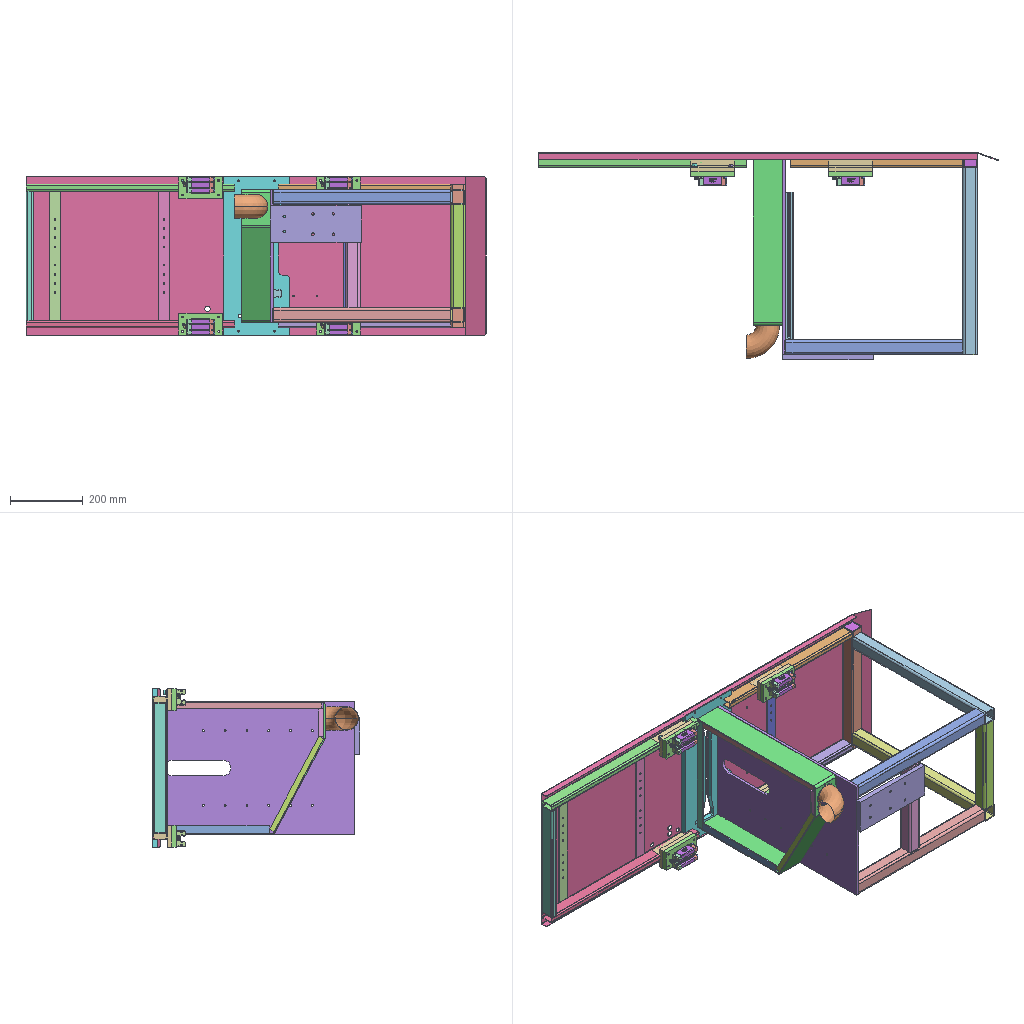Assembly | SolidWorks | 13 different items | 23 placed | box 1267 x 570 x 440 mm
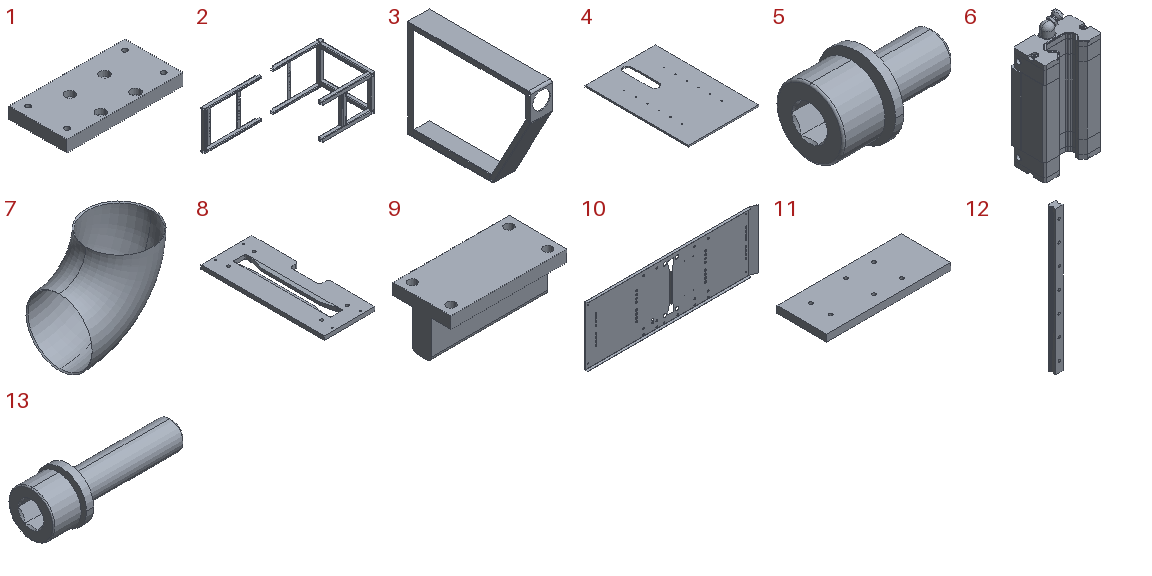Parts list (item | quantity | size | volume | features):
1 | x4 | 120 x 60 x 12 mm | 83068 mm3 | features HoleWzd 2, 3DProfileFeature 1, Extrusion 1
2 | x1 | 1210 x 555 x 396 mm | 2067194 mm3 | features ICE 3, WeldMemberFeat 3, WeldCornerFeat 2, 3DProfileFeature 1, EndCap 1, HoleWzd 1, WeldmentFeature 1
3 | x1 | 80 x 460 x 365 mm | 345434 mm3 | features ICE 3, FlatPattern 1, SMBaseFlange 1, SheetMetal 1
4 | x1 | 365 x 540 x 8 mm | 1513471 mm3 | features Extrusion 1, HoleWzd 1, LPattern 1
5 | x1 | 24 x 15 x 15 mm | 1870 mm3 | features RevCut 2, Revolution 2, Chamfer 1, Cut 1, Fillet 1
6 | x4 | 44.1 x 25.7 x 88.625 mm | 65252 mm3 | features ICE 20, Extrusion 4, MirrorPattern 4, Chamfer 3, Fillet 3, MirrorSolid 3, Revolution 2, Dome 1, RevCut 1
7 | x1 | 91.534 x 65 x 91.534 mm | 19075 mm3 | features Chamfer 1, Revolution 1
8 | x1 | 180 x 436 x 14 mm | 907497 mm3 | features HoleWzd 2, ICE 2, Extrusion 1, Fillet 1
9 | x4 | 120 x 60 x 52 mm | 178059 mm3 | features Extrusion 1, Fillet 1, HoleWzd 1, ICE 1
10 | x1 | 1267 x 21.649 x 440.4 mm | 706056 mm3 | features EdgeFlange 3, HoleWzd 3, LPattern 3, Fillet 2, ICE 2, FlatPattern 1, SMBaseFlange 1, SheetMetal 1
11 | x1 | 250 x 100 x 14 mm | 346949 mm3 | features HoleWzd 2, Extrusion 1
12 | x2 | 23 x 22 x 420 mm | 180087 mm3 | features ICE 17, Chamfer 3, Extrusion 3, Fillet 3, MirrorPattern 3, MirrorSolid 3, RevCut 2, DeleteBody 1, Dome 1, LPattern 1
13 | x1 | 31 x 11 x 11 mm | 1178 mm3 | features RevCut 2, Revolution 2, Chamfer 1, Cut 1, Fillet 1
Mates (type | each side: item.copy, entity, surface, feature):
DistanceDim | 9.1 face plane Boss-Extrude1 | 9.2 face plane Boss-Extrude1
Coincident | 2.1 face plane Cut-Extrude2 | 8.1 face plane Boss-Extrude1 | 2 times
Coincident | 8.1 face plane Boss-Extrude1 | 4.1 face plane Boss-Extrude1
Coincident | 9.1 face plane Boss-Extrude1 | 9.3 face plane Boss-Extrude1 | 2 times
Coincident | 4.1 face plane Boss-Extrude1 | 3.1 face plane Base-Flange1 | 2 times
Coincident | 8.1 face plane Boss-Extrude1 | 3.1 face plane Base-Flange1
DistanceDim | 3.1 face plane Base-Flange1 | 7.1 plane
Coincident | 2.1 face plane Square Tube 40 X 40 X 3.2(1) | 11.1 face plane Boss-Extrude1
Coincident | 4.1 face plane Boss-Extrude1 | 11.1 face plane Boss-Extrude1
DistanceDim | 11.1 face plane Boss-Extrude1 | 2.1 face plane Square Tube 40 X 40 X 3.2(1)
Concentric | assembly face | 1.1 face cylinder Hole Size (per hex socket screw type)1
Concentric | assembly face | 1.1 edge
Coincident | assembly face | 1.1 face plane Boss-Extrude1
Coincident | 9.3 face plane Boss-Extrude1 | 1.1 face plane Boss-Extrude1 | 3 times
Concentric | assembly face | 1.2 edge
Concentric | assembly edge | 1.2 face cylinder Hole Size (per hex socket screw type)1
Coincident | assembly face | 1.2 face plane Boss-Extrude1
Coincident | 9.1 face plane Boss-Extrude1 | 1.2 face plane Boss-Extrude1 | 3 times
Coincident | 9.2 face plane Boss-Extrude1 | 1.3 face plane Boss-Extrude1 | 3 times
Coincident | 9.4 face plane Boss-Extrude1 | 1.4 face plane Boss-Extrude1 | 3 times
Coincident | 8.1 face plane Boss-Extrude1 | 10.1 face plane Base-Flange1
Coincident | 4.1 face plane Boss-Extrude1 | 12.1 face plane Boss-Extrude8
Width | 3.1 face plane Base-Flange1 | 3.1 face plane Base-Flange1 | 8.1 face plane Boss-Extrude1 | 8.1 face plane Boss-Extrude1
Coincident | 1.4 face plane Boss-Extrude1 | 1.3 face plane Boss-Extrude1
Coincident | 9.1 face plane Boss-Extrude1 | 9.2 face plane Boss-Extrude1
Concentric | 1.1 edge | 6.1 face cylinder Cut-Revolve1
Concentric | 1.1 face cylinder Hole Size (per hex socket screw type)1 | 6.1 face cylinder Mirror1
Coincident | 1.1 face plane Boss-Extrude1 | 6.1 face plane Boss-Extrude1
Concentric | 1.2 edge | 6.2 face cylinder Cut-Revolve1
Concentric | 1.2 face cylinder Hole Size (per hex socket screw type)1 | 6.2 face cylinder Mirror2
Coincident | 1.2 face plane Boss-Extrude1 | 6.2 face plane Boss-Extrude1
Concentric | 1.3 face cylinder Hole Size (per hex socket screw type)1 | 6.3 face cylinder Mirror2
Concentric | 1.3 edge | 6.3 face cylinder Cut-Revolve1
Coincident | 1.3 face plane Boss-Extrude1 | 6.3 face plane Boss-Extrude1
Concentric | 1.4 face cylinder Hole Size (per hex socket screw type)1 | 6.4 face cylinder Cut-Revolve1
Concentric | 1.4 face cylinder Hole Size (per hex socket screw type)1 | 6.4 face cylinder Mirror1
Coincident | 1.4 face plane Boss-Extrude1 | 6.4 face plane Boss-Extrude1
Coincident | 9.4 face plane Boss-Extrude1 | 9.3 face plane Boss-Extrude1 | 2 times
Concentric | 4.1 face cylinder LPattern1 | 12.1 face cylinder LPattern1
Concentric | 4.1 face cylinder LPattern1 | 12.2 face cylinder LPattern1
Width | 8.1 face plane Boss-Extrude1 | 8.1 face plane Boss-Extrude1 | 2.1 face plane Rect Tube 40X20X2.5(6) | 2.1 face plane Rect Tube 40X20X2.5(6)
DistanceDim | 4.1 face plane Boss-Extrude1 | 8.1 face plane Boss-Extrude1
Coincident | 2.1 face plane Rect Tube 40X20X2.5(6) | 9.1 face plane Boss-Extrude2
Coincident | 2.1 face plane Rect Tube 40X20X2.5(6) | 9.3 face plane Boss-Extrude2
Coincident | 9.4 face plane Boss-Extrude1 | 9.2 face plane Boss-Extrude1
DistanceDim | 1.3 face plane Boss-Extrude1 | 4.1 face plane Boss-Extrude1
Coincident | 2.1 face plane Rect Tube 40X20X2.5(6) | 9.1 face plane Boss-Extrude1
Concentric | 8.1 face cylinder M12 Tapped Hole1 | 10.1 face cylinder Base-Flange1 | 2 times
Coincident | 3.1 face plane Base-Flange1 | 7.1 plane
DistanceDim | 7.1 plane | 4.1 face plane Boss-Extrude1
Coincident | 12.1 face plane Boss-Extrude8 | 12.2 face plane Boss-Extrude8
Coincident | 12.1 face plane Cut-Extrude13 | 12.2 face plane Cut-Extrude13
Coincident | 9.1 face plane Boss-Extrude1 | 5.1 face plane Revolve1
Concentric | 9.1 face cylinder M6 Clearance Hole1 | 5.1 face cylinder Base-Revolve
Coincident | 9.1 face plane Boss-Extrude1 | 13.1 face plane Revolve1
Concentric | 9.1 face cylinder M6 Clearance Hole1 | 13.1 face cylinder Base-Revolve